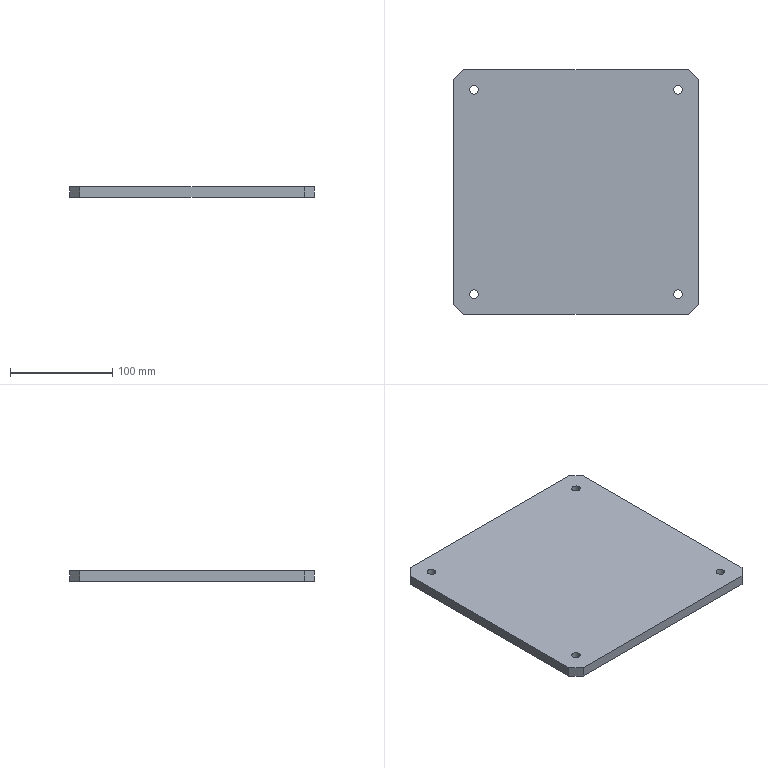Part | STEP file | PN_0011 | 1 solid | 18 faces | box 240 x 240 x 10 mm | volume 571730 mm3 | plane 10 | cylinder 8 | commonest cylinder face diameters 8.5 x8
STEP:
#1=CARTESIAN_POINT('',(0.,0.,0.));
#2=DIRECTION('',(0.,0.,1.));
#3=DIRECTION('',(1.,0.,0.));
#4=AXIS2_PLACEMENT_3D('',#1,#2,#3);
#5=CARTESIAN_POINT('',(-95.75,100.,0.));
#6=VERTEX_POINT('',#5);
#7=CARTESIAN_POINT('',(-95.75,100.,10.));
#8=VERTEX_POINT('',#7);
#9=CARTESIAN_POINT('',(-95.75,100.,10.));
#10=DIRECTION('',(0.,0.,1.));
#11=VECTOR('',#10,1.);
#12=LINE('',#9,#11);
#13=CARTESIAN_POINT('',(-100.,100.,10.));
#14=DIRECTION('',(0.,0.,1.));
#15=DIRECTION('',(1.,0.,0.));
#16=AXIS2_PLACEMENT_3D('',#13,#14,#15);
#17=CYLINDRICAL_SURFACE('',#16,4.25);
#18=CARTESIAN_POINT('',(6.283,0.));
#19=DIRECTION('',(0.,1.));
#20=VECTOR('',#19,1.);
#21=LINE('',#18,#20);
#22=(GEOMETRIC_REPRESENTATION_CONTEXT(2)PARAMETRIC_REPRESENTATION_CONTEXT()REPRESENTATION_CONTEXT('',''));
#23=DEFINITIONAL_REPRESENTATION('',(#21),#22);
#24=PCURVE('',#17,#23);
#25=CARTESIAN_POINT('',(-100.,100.,10.));
#26=DIRECTION('',(0.,0.,1.));
#27=DIRECTION('',(1.,0.,0.));
#28=AXIS2_PLACEMENT_3D('',#25,#26,#27);
#29=CYLINDRICAL_SURFACE('',#28,4.25);
#30=CARTESIAN_POINT('',(0.,0.));
#31=DIRECTION('',(0.,1.));
#32=VECTOR('',#31,1.);
#33=LINE('',#30,#32);
#34=(GEOMETRIC_REPRESENTATION_CONTEXT(2)PARAMETRIC_REPRESENTATION_CONTEXT()REPRESENTATION_CONTEXT('',''));
#35=DEFINITIONAL_REPRESENTATION('',(#33),#34);
#36=PCURVE('',#29,#35);
#37=SURFACE_CURVE('',#12,(#24,#36),.PCURVE_S1.);
#38=EDGE_CURVE('',#6,#8,#37,.T.);
#39=ORIENTED_EDGE('',*,*,#38,.T.);
#40=CARTESIAN_POINT('',(-104.25,100.,10.));
#41=VERTEX_POINT('',#40);
#42=CARTESIAN_POINT('',(-100.,100.,10.));
#43=DIRECTION('',(0.,0.,1.));
#44=DIRECTION('',(1.,0.,0.));
#45=AXIS2_PLACEMENT_3D('',#42,#43,#44);
#46=CIRCLE('',#45,4.25);
#47=CARTESIAN_POINT('',(0.,0.));
#48=DIRECTION('',(1.,0.));
#49=VECTOR('',#48,1.);
#50=LINE('',#47,#49);
#51=(GEOMETRIC_REPRESENTATION_CONTEXT(2)PARAMETRIC_REPRESENTATION_CONTEXT()REPRESENTATION_CONTEXT('',''));
#52=DEFINITIONAL_REPRESENTATION('',(#50),#51);
#53=PCURVE('',#17,#52);
#54=CARTESIAN_POINT('',(0.,0.,10.));
#55=DIRECTION('',(0.,0.,1.));
#56=DIRECTION('',(1.,0.,0.));
#57=AXIS2_PLACEMENT_3D('',#54,#55,#56);
#58=PLANE('',#57);
#59=CARTESIAN_POINT('',(-100.,100.));
#60=DIRECTION('',(1.,0.));
#61=AXIS2_PLACEMENT_2D('',#59,#60);
#62=CIRCLE('',#61,4.25);
#63=(GEOMETRIC_REPRESENTATION_CONTEXT(2)PARAMETRIC_REPRESENTATION_CONTEXT()REPRESENTATION_CONTEXT('',''));
#64=DEFINITIONAL_REPRESENTATION('',(#62),#63);
#65=PCURVE('',#58,#64);
#66=SURFACE_CURVE('',#46,(#53,#65),.PCURVE_S1.);
#67=EDGE_CURVE('',#41,#8,#66,.T.);
#68=ORIENTED_EDGE('',*,*,#67,.F.);
#69=CARTESIAN_POINT('',(-104.25,100.,0.));
#70=VERTEX_POINT('',#69);
#71=CARTESIAN_POINT('',(-104.25,100.,10.));
#72=DIRECTION('',(0.,0.,1.));
#73=VECTOR('',#72,1.);
#74=LINE('',#71,#73);
#75=CARTESIAN_POINT('',(3.142,0.));
#76=DIRECTION('',(0.,1.));
#77=VECTOR('',#76,1.);
#78=LINE('',#75,#77);
#79=(GEOMETRIC_REPRESENTATION_CONTEXT(2)PARAMETRIC_REPRESENTATION_CONTEXT()REPRESENTATION_CONTEXT('',''));
#80=DEFINITIONAL_REPRESENTATION('',(#78),#79);
#81=PCURVE('',#17,#80);
#82=CARTESIAN_POINT('',(3.142,0.));
#83=DIRECTION('',(0.,1.));
#84=VECTOR('',#83,1.);
#85=LINE('',#82,#84);
#86=(GEOMETRIC_REPRESENTATION_CONTEXT(2)PARAMETRIC_REPRESENTATION_CONTEXT()REPRESENTATION_CONTEXT('',''));
#87=DEFINITIONAL_REPRESENTATION('',(#85),#86);
#88=PCURVE('',#29,#87);
#89=SURFACE_CURVE('',#74,(#81,#88),.PCURVE_S1.);
#90=EDGE_CURVE('',#70,#41,#89,.T.);
#91=ORIENTED_EDGE('',*,*,#90,.F.);
#92=CARTESIAN_POINT('',(-100.,100.,0.));
#93=DIRECTION('',(0.,0.,1.));
#94=DIRECTION('',(1.,0.,0.));
#95=AXIS2_PLACEMENT_3D('',#92,#93,#94);
#96=CIRCLE('',#95,4.25);
#97=CARTESIAN_POINT('',(0.,-10.));
#98=DIRECTION('',(1.,0.));
#99=VECTOR('',#98,1.);
#100=LINE('',#97,#99);
#101=(GEOMETRIC_REPRESENTATION_CONTEXT(2)PARAMETRIC_REPRESENTATION_CONTEXT()REPRESENTATION_CONTEXT('',''));
#102=DEFINITIONAL_REPRESENTATION('',(#100),#101);
#103=PCURVE('',#17,#102);
#104=CARTESIAN_POINT('',(0.,0.,0.));
#105=DIRECTION('',(0.,0.,1.));
#106=DIRECTION('',(1.,0.,0.));
#107=AXIS2_PLACEMENT_3D('',#104,#105,#106);
#108=PLANE('',#107);
#109=CARTESIAN_POINT('',(-100.,100.));
#110=DIRECTION('',(1.,0.));
#111=AXIS2_PLACEMENT_2D('',#109,#110);
#112=CIRCLE('',#111,4.25);
#113=(GEOMETRIC_REPRESENTATION_CONTEXT(2)PARAMETRIC_REPRESENTATION_CONTEXT()REPRESENTATION_CONTEXT('',''));
#114=DEFINITIONAL_REPRESENTATION('',(#112),#113);
#115=PCURVE('',#108,#114);
#116=SURFACE_CURVE('',#96,(#103,#115),.PCURVE_S1.);
#117=EDGE_CURVE('',#70,#6,#116,.T.);
#118=ORIENTED_EDGE('',*,*,#117,.T.);
#119=EDGE_LOOP('',(#39,#68,#91,#118));
#120=FACE_BOUND('',#119,.F.);
#121=ADVANCED_FACE('',(#120),#17,.F.);
#122=CARTESIAN_POINT('',(-95.75,-100.,0.));
#123=VERTEX_POINT('',#122);
#124=CARTESIAN_POINT('',(-95.75,-100.,10.));
#125=VERTEX_POINT('',#124);
#126=CARTESIAN_POINT('',(-95.75,-100.,10.));
#127=DIRECTION('',(0.,0.,1.));
#128=VECTOR('',#127,1.);
#129=LINE('',#126,#128);
#130=CARTESIAN_POINT('',(-100.,-100.,10.));
#131=DIRECTION('',(0.,0.,1.));
#132=DIRECTION('',(1.,0.,0.));
#133=AXIS2_PLACEMENT_3D('',#130,#131,#132);
#134=CYLINDRICAL_SURFACE('',#133,4.25);
#135=CARTESIAN_POINT('',(6.283,0.));
#136=DIRECTION('',(0.,1.));
#137=VECTOR('',#136,1.);
#138=LINE('',#135,#137);
#139=(GEOMETRIC_REPRESENTATION_CONTEXT(2)PARAMETRIC_REPRESENTATION_CONTEXT()REPRESENTATION_CONTEXT('',''));
#140=DEFINITIONAL_REPRESENTATION('',(#138),#139);
#141=PCURVE('',#134,#140);
#142=CARTESIAN_POINT('',(-100.,-100.,10.));
#143=DIRECTION('',(0.,0.,1.));
#144=DIRECTION('',(1.,0.,0.));
#145=AXIS2_PLACEMENT_3D('',#142,#143,#144);
#146=CYLINDRICAL_SURFACE('',#145,4.25);
#147=CARTESIAN_POINT('',(0.,0.));
#148=DIRECTION('',(0.,1.));
#149=VECTOR('',#148,1.);
#150=LINE('',#147,#149);
#151=(GEOMETRIC_REPRESENTATION_CONTEXT(2)PARAMETRIC_REPRESENTATION_CONTEXT()REPRESENTATION_CONTEXT('',''));
#152=DEFINITIONAL_REPRESENTATION('',(#150),#151);
#153=PCURVE('',#146,#152);
#154=SURFACE_CURVE('',#129,(#141,#153),.PCURVE_S1.);
#155=EDGE_CURVE('',#123,#125,#154,.T.);
#156=ORIENTED_EDGE('',*,*,#155,.T.);
#157=CARTESIAN_POINT('',(-104.25,-100.,10.));
#158=VERTEX_POINT('',#157);
#159=CARTESIAN_POINT('',(-100.,-100.,10.));
#160=DIRECTION('',(0.,0.,1.));
#161=DIRECTION('',(1.,0.,0.));
#162=AXIS2_PLACEMENT_3D('',#159,#160,#161);
#163=CIRCLE('',#162,4.25);
#164=CARTESIAN_POINT('',(0.,0.));
#165=DIRECTION('',(1.,0.));
#166=VECTOR('',#165,1.);
#167=LINE('',#164,#166);
#168=(GEOMETRIC_REPRESENTATION_CONTEXT(2)PARAMETRIC_REPRESENTATION_CONTEXT()REPRESENTATION_CONTEXT('',''));
#169=DEFINITIONAL_REPRESENTATION('',(#167),#168);
#170=PCURVE('',#134,#169);
#171=CARTESIAN_POINT('',(-100.,-100.));
#172=DIRECTION('',(1.,0.));
#173=AXIS2_PLACEMENT_2D('',#171,#172);
#174=CIRCLE('',#173,4.25);
#175=(GEOMETRIC_REPRESENTATION_CONTEXT(2)PARAMETRIC_REPRESENTATION_CONTEXT()REPRESENTATION_CONTEXT('',''));
#176=DEFINITIONAL_REPRESENTATION('',(#174),#175);
#177=PCURVE('',#58,#176);
#178=SURFACE_CURVE('',#163,(#170,#177),.PCURVE_S1.);
#179=EDGE_CURVE('',#158,#125,#178,.T.);
#180=ORIENTED_EDGE('',*,*,#179,.F.);
#181=CARTESIAN_POINT('',(-104.25,-100.,0.));
#182=VERTEX_POINT('',#181);
#183=CARTESIAN_POINT('',(-104.25,-100.,10.));
#184=DIRECTION('',(0.,0.,1.));
#185=VECTOR('',#184,1.);
#186=LINE('',#183,#185);
#187=CARTESIAN_POINT('',(3.142,0.));
#188=DIRECTION('',(0.,1.));
#189=VECTOR('',#188,1.);
#190=LINE('',#187,#189);
#191=(GEOMETRIC_REPRESENTATION_CONTEXT(2)PARAMETRIC_REPRESENTATION_CONTEXT()REPRESENTATION_CONTEXT('',''));
#192=DEFINITIONAL_REPRESENTATION('',(#190),#191);
#193=PCURVE('',#134,#192);
#194=CARTESIAN_POINT('',(3.142,0.));
#195=DIRECTION('',(0.,1.));
#196=VECTOR('',#195,1.);
#197=LINE('',#194,#196);
#198=(GEOMETRIC_REPRESENTATION_CONTEXT(2)PARAMETRIC_REPRESENTATION_CONTEXT()REPRESENTATION_CONTEXT('',''));
#199=DEFINITIONAL_REPRESENTATION('',(#197),#198);
#200=PCURVE('',#146,#199);
#201=SURFACE_CURVE('',#186,(#193,#200),.PCURVE_S1.);
#202=EDGE_CURVE('',#182,#158,#201,.T.);
#203=ORIENTED_EDGE('',*,*,#202,.F.);
#204=CARTESIAN_POINT('',(-100.,-100.,0.));
#205=DIRECTION('',(0.,0.,1.));
#206=DIRECTION('',(1.,0.,0.));
#207=AXIS2_PLACEMENT_3D('',#204,#205,#206);
#208=CIRCLE('',#207,4.25);
#209=CARTESIAN_POINT('',(0.,-10.));
#210=DIRECTION('',(1.,0.));
#211=VECTOR('',#210,1.);
#212=LINE('',#209,#211);
#213=(GEOMETRIC_REPRESENTATION_CONTEXT(2)PARAMETRIC_REPRESENTATION_CONTEXT()REPRESENTATION_CONTEXT('',''));
#214=DEFINITIONAL_REPRESENTATION('',(#212),#213);
#215=PCURVE('',#134,#214);
#216=CARTESIAN_POINT('',(-100.,-100.));
#217=DIRECTION('',(1.,0.));
#218=AXIS2_PLACEMENT_2D('',#216,#217);
#219=CIRCLE('',#218,4.25);
#220=(GEOMETRIC_REPRESENTATION_CONTEXT(2)PARAMETRIC_REPRESENTATION_CONTEXT()REPRESENTATION_CONTEXT('',''));
#221=DEFINITIONAL_REPRESENTATION('',(#219),#220);
#222=PCURVE('',#108,#221);
#223=SURFACE_CURVE('',#208,(#215,#222),.PCURVE_S1.);
#224=EDGE_CURVE('',#182,#123,#223,.T.);
#225=ORIENTED_EDGE('',*,*,#224,.T.);
#226=EDGE_LOOP('',(#156,#180,#203,#225));
#227=FACE_BOUND('',#226,.F.);
#228=ADVANCED_FACE('',(#227),#134,.F.);
#229=CARTESIAN_POINT('',(104.25,100.,0.));
#230=VERTEX_POINT('',#229);
#231=CARTESIAN_POINT('',(104.25,100.,10.));
#232=VERTEX_POINT('',#231);
#233=CARTESIAN_POINT('',(104.25,100.,10.));
#234=DIRECTION('',(0.,0.,1.));
#235=VECTOR('',#234,1.);
#236=LINE('',#233,#235);
#237=CARTESIAN_POINT('',(100.,100.,10.));
#238=DIRECTION('',(0.,0.,1.));
#239=DIRECTION('',(1.,0.,0.));
#240=AXIS2_PLACEMENT_3D('',#237,#238,#239);
#241=CYLINDRICAL_SURFACE('',#240,4.25);
#242=CARTESIAN_POINT('',(6.283,0.));
#243=DIRECTION('',(0.,1.));
#244=VECTOR('',#243,1.);
#245=LINE('',#242,#244);
#246=(GEOMETRIC_REPRESENTATION_CONTEXT(2)PARAMETRIC_REPRESENTATION_CONTEXT()REPRESENTATION_CONTEXT('',''));
#247=DEFINITIONAL_REPRESENTATION('',(#245),#246);
#248=PCURVE('',#241,#247);
#249=CARTESIAN_POINT('',(100.,100.,10.));
#250=DIRECTION('',(0.,0.,1.));
#251=DIRECTION('',(1.,0.,0.));
#252=AXIS2_PLACEMENT_3D('',#249,#250,#251);
#253=CYLINDRICAL_SURFACE('',#252,4.25);
#254=CARTESIAN_POINT('',(0.,0.));
#255=DIRECTION('',(0.,1.));
#256=VECTOR('',#255,1.);
#257=LINE('',#254,#256);
#258=(GEOMETRIC_REPRESENTATION_CONTEXT(2)PARAMETRIC_REPRESENTATION_CONTEXT()REPRESENTATION_CONTEXT('',''));
#259=DEFINITIONAL_REPRESENTATION('',(#257),#258);
#260=PCURVE('',#253,#259);
#261=SURFACE_CURVE('',#236,(#248,#260),.PCURVE_S1.);
#262=EDGE_CURVE('',#230,#232,#261,.T.);
#263=ORIENTED_EDGE('',*,*,#262,.T.);
#264=CARTESIAN_POINT('',(95.75,100.,10.));
#265=VERTEX_POINT('',#264);
#266=CARTESIAN_POINT('',(100.,100.,10.));
#267=DIRECTION('',(0.,0.,1.));
#268=DIRECTION('',(1.,0.,0.));
#269=AXIS2_PLACEMENT_3D('',#266,#267,#268);
#270=CIRCLE('',#269,4.25);
#271=CARTESIAN_POINT('',(0.,0.));
#272=DIRECTION('',(1.,0.));
#273=VECTOR('',#272,1.);
#274=LINE('',#271,#273);
#275=(GEOMETRIC_REPRESENTATION_CONTEXT(2)PARAMETRIC_REPRESENTATION_CONTEXT()REPRESENTATION_CONTEXT('',''));
#276=DEFINITIONAL_REPRESENTATION('',(#274),#275);
#277=PCURVE('',#241,#276);
#278=CARTESIAN_POINT('',(100.,100.));
#279=DIRECTION('',(1.,0.));
#280=AXIS2_PLACEMENT_2D('',#278,#279);
#281=CIRCLE('',#280,4.25);
#282=(GEOMETRIC_REPRESENTATION_CONTEXT(2)PARAMETRIC_REPRESENTATION_CONTEXT()REPRESENTATION_CONTEXT('',''));
#283=DEFINITIONAL_REPRESENTATION('',(#281),#282);
#284=PCURVE('',#58,#283);
#285=SURFACE_CURVE('',#270,(#277,#284),.PCURVE_S1.);
#286=EDGE_CURVE('',#265,#232,#285,.T.);
#287=ORIENTED_EDGE('',*,*,#286,.F.);
#288=CARTESIAN_POINT('',(95.75,100.,0.));
#289=VERTEX_POINT('',#288);
#290=CARTESIAN_POINT('',(95.75,100.,10.));
#291=DIRECTION('',(0.,0.,1.));
#292=VECTOR('',#291,1.);
#293=LINE('',#290,#292);
#294=CARTESIAN_POINT('',(3.142,0.));
#295=DIRECTION('',(0.,1.));
#296=VECTOR('',#295,1.);
#297=LINE('',#294,#296);
#298=(GEOMETRIC_REPRESENTATION_CONTEXT(2)PARAMETRIC_REPRESENTATION_CONTEXT()REPRESENTATION_CONTEXT('',''));
#299=DEFINITIONAL_REPRESENTATION('',(#297),#298);
#300=PCURVE('',#241,#299);
#301=CARTESIAN_POINT('',(3.142,0.));
#302=DIRECTION('',(0.,1.));
#303=VECTOR('',#302,1.);
#304=LINE('',#301,#303);
#305=(GEOMETRIC_REPRESENTATION_CONTEXT(2)PARAMETRIC_REPRESENTATION_CONTEXT()REPRESENTATION_CONTEXT('',''));
#306=DEFINITIONAL_REPRESENTATION('',(#304),#305);
#307=PCURVE('',#253,#306);
#308=SURFACE_CURVE('',#293,(#300,#307),.PCURVE_S1.);
#309=EDGE_CURVE('',#289,#265,#308,.T.);
#310=ORIENTED_EDGE('',*,*,#309,.F.);
#311=CARTESIAN_POINT('',(100.,100.,0.));
#312=DIRECTION('',(0.,0.,1.));
#313=DIRECTION('',(1.,0.,0.));
#314=AXIS2_PLACEMENT_3D('',#311,#312,#313);
#315=CIRCLE('',#314,4.25);
#316=CARTESIAN_POINT('',(0.,-10.));
#317=DIRECTION('',(1.,0.));
#318=VECTOR('',#317,1.);
#319=LINE('',#316,#318);
#320=(GEOMETRIC_REPRESENTATION_CONTEXT(2)PARAMETRIC_REPRESENTATION_CONTEXT()REPRESENTATION_CONTEXT('',''));
#321=DEFINITIONAL_REPRESENTATION('',(#319),#320);
#322=PCURVE('',#241,#321);
#323=CARTESIAN_POINT('',(100.,100.));
#324=DIRECTION('',(1.,0.));
#325=AXIS2_PLACEMENT_2D('',#323,#324);
#326=CIRCLE('',#325,4.25);
#327=(GEOMETRIC_REPRESENTATION_CONTEXT(2)PARAMETRIC_REPRESENTATION_CONTEXT()REPRESENTATION_CONTEXT('',''));
#328=DEFINITIONAL_REPRESENTATION('',(#326),#327);
#329=PCURVE('',#108,#328);
#330=SURFACE_CURVE('',#315,(#322,#329),.PCURVE_S1.);
#331=EDGE_CURVE('',#289,#230,#330,.T.);
#332=ORIENTED_EDGE('',*,*,#331,.T.);
#333=EDGE_LOOP('',(#263,#287,#310,#332));
#334=FACE_BOUND('',#333,.F.);
#335=ADVANCED_FACE('',(#334),#241,.F.);
#336=CARTESIAN_POINT('',(104.25,-100.,0.));
#337=VERTEX_POINT('',#336);
#338=CARTESIAN_POINT('',(104.25,-100.,10.));
#339=VERTEX_POINT('',#338);
#340=CARTESIAN_POINT('',(104.25,-100.,10.));
#341=DIRECTION('',(0.,0.,1.));
#342=VECTOR('',#341,1.);
#343=LINE('',#340,#342);
#344=CARTESIAN_POINT('',(100.,-100.,10.));
#345=DIRECTION('',(0.,0.,1.));
#346=DIRECTION('',(1.,0.,0.));
#347=AXIS2_PLACEMENT_3D('',#344,#345,#346);
#348=CYLINDRICAL_SURFACE('',#347,4.25);
#349=CARTESIAN_POINT('',(6.283,0.));
#350=DIRECTION('',(0.,1.));
#351=VECTOR('',#350,1.);
#352=LINE('',#349,#351);
#353=(GEOMETRIC_REPRESENTATION_CONTEXT(2)PARAMETRIC_REPRESENTATION_CONTEXT()REPRESENTATION_CONTEXT('',''));
#354=DEFINITIONAL_REPRESENTATION('',(#352),#353);
#355=PCURVE('',#348,#354);
#356=CARTESIAN_POINT('',(100.,-100.,10.));
#357=DIRECTION('',(0.,0.,1.));
#358=DIRECTION('',(1.,0.,0.));
#359=AXIS2_PLACEMENT_3D('',#356,#357,#358);
#360=CYLINDRICAL_SURFACE('',#359,4.25);
#361=CARTESIAN_POINT('',(0.,0.));
#362=DIRECTION('',(0.,1.));
#363=VECTOR('',#362,1.);
#364=LINE('',#361,#363);
#365=(GEOMETRIC_REPRESENTATION_CONTEXT(2)PARAMETRIC_REPRESENTATION_CONTEXT()REPRESENTATION_CONTEXT('',''));
#366=DEFINITIONAL_REPRESENTATION('',(#364),#365);
#367=PCURVE('',#360,#366);
#368=SURFACE_CURVE('',#343,(#355,#367),.PCURVE_S1.);
#369=EDGE_CURVE('',#337,#339,#368,.T.);
#370=ORIENTED_EDGE('',*,*,#369,.T.);
#371=CARTESIAN_POINT('',(95.75,-100.,10.));
#372=VERTEX_POINT('',#371);
#373=CARTESIAN_POINT('',(100.,-100.,10.));
#374=DIRECTION('',(0.,0.,1.));
#375=DIRECTION('',(1.,0.,0.));
#376=AXIS2_PLACEMENT_3D('',#373,#374,#375);
#377=CIRCLE('',#376,4.25);
#378=CARTESIAN_POINT('',(0.,0.));
#379=DIRECTION('',(1.,0.));
#380=VECTOR('',#379,1.);
#381=LINE('',#378,#380);
#382=(GEOMETRIC_REPRESENTATION_CONTEXT(2)PARAMETRIC_REPRESENTATION_CONTEXT()REPRESENTATION_CONTEXT('',''));
#383=DEFINITIONAL_REPRESENTATION('',(#381),#382);
#384=PCURVE('',#348,#383);
#385=CARTESIAN_POINT('',(100.,-100.));
#386=DIRECTION('',(1.,0.));
#387=AXIS2_PLACEMENT_2D('',#385,#386);
#388=CIRCLE('',#387,4.25);
#389=(GEOMETRIC_REPRESENTATION_CONTEXT(2)PARAMETRIC_REPRESENTATION_CONTEXT()REPRESENTATION_CONTEXT('',''));
#390=DEFINITIONAL_REPRESENTATION('',(#388),#389);
#391=PCURVE('',#58,#390);
#392=SURFACE_CURVE('',#377,(#384,#391),.PCURVE_S1.);
#393=EDGE_CURVE('',#372,#339,#392,.T.);
#394=ORIENTED_EDGE('',*,*,#393,.F.);
#395=CARTESIAN_POINT('',(95.75,-100.,0.));
#396=VERTEX_POINT('',#395);
#397=CARTESIAN_POINT('',(95.75,-100.,10.));
#398=DIRECTION('',(0.,0.,1.));
#399=VECTOR('',#398,1.);
#400=LINE('',#397,#399);
#401=CARTESIAN_POINT('',(3.142,0.));
#402=DIRECTION('',(0.,1.));
#403=VECTOR('',#402,1.);
#404=LINE('',#401,#403);
#405=(GEOMETRIC_REPRESENTATION_CONTEXT(2)PARAMETRIC_REPRESENTATION_CONTEXT()REPRESENTATION_CONTEXT('',''));
#406=DEFINITIONAL_REPRESENTATION('',(#404),#405);
#407=PCURVE('',#348,#406);
#408=CARTESIAN_POINT('',(3.142,0.));
#409=DIRECTION('',(0.,1.));
#410=VECTOR('',#409,1.);
#411=LINE('',#408,#410);
#412=(GEOMETRIC_REPRESENTATION_CONTEXT(2)PARAMETRIC_REPRESENTATION_CONTEXT()REPRESENTATION_CONTEXT('',''));
#413=DEFINITIONAL_REPRESENTATION('',(#411),#412);
#414=PCURVE('',#360,#413);
#415=SURFACE_CURVE('',#400,(#407,#414),.PCURVE_S1.);
#416=EDGE_CURVE('',#396,#372,#415,.T.);
#417=ORIENTED_EDGE('',*,*,#416,.F.);
#418=CARTESIAN_POINT('',(100.,-100.,0.));
#419=DIRECTION('',(0.,0.,1.));
#420=DIRECTION('',(1.,0.,0.));
#421=AXIS2_PLACEMENT_3D('',#418,#419,#420);
#422=CIRCLE('',#421,4.25);
#423=CARTESIAN_POINT('',(0.,-10.));
#424=DIRECTION('',(1.,0.));
#425=VECTOR('',#424,1.);
#426=LINE('',#423,#425);
#427=(GEOMETRIC_REPRESENTATION_CONTEXT(2)PARAMETRIC_REPRESENTATION_CONTEXT()REPRESENTATION_CONTEXT('',''));
#428=DEFINITIONAL_REPRESENTATION('',(#426),#427);
#429=PCURVE('',#348,#428);
#430=CARTESIAN_POINT('',(100.,-100.));
#431=DIRECTION('',(1.,0.));
#432=AXIS2_PLACEMENT_2D('',#430,#431);
#433=CIRCLE('',#432,4.25);
#434=(GEOMETRIC_REPRESENTATION_CONTEXT(2)PARAMETRIC_REPRESENTATION_CONTEXT()REPRESENTATION_CONTEXT('',''));
#435=DEFINITIONAL_REPRESENTATION('',(#433),#434);
#436=PCURVE('',#108,#435);
#437=SURFACE_CURVE('',#422,(#429,#436),.PCURVE_S1.);
#438=EDGE_CURVE('',#396,#337,#437,.T.);
#439=ORIENTED_EDGE('',*,*,#438,.T.);
#440=EDGE_LOOP('',(#370,#394,#417,#439));
#441=FACE_BOUND('',#440,.F.);
#442=ADVANCED_FACE('',(#441),#348,.F.);
#443=CARTESIAN_POINT('',(120.,-110.,0.));
#444=VERTEX_POINT('',#443);
#445=CARTESIAN_POINT('',(120.,110.,0.));
#446=VERTEX_POINT('',#445);
#447=CARTESIAN_POINT('',(120.,120.,0.));
#448=DIRECTION('',(0.,1.,0.));
#449=VECTOR('',#448,1.);
#450=LINE('',#447,#449);
#451=CARTESIAN_POINT('',(120.,120.,10.));
#452=DIRECTION('',(-1.,0.,0.));
#453=DIRECTION('',(0.,-1.,0.));
#454=AXIS2_PLACEMENT_3D('',#451,#452,#453);
#455=PLANE('',#454);
#456=CARTESIAN_POINT('',(0.,-10.));
#457=DIRECTION('',(-1.,0.));
#458=VECTOR('',#457,1.);
#459=LINE('',#456,#458);
#460=(GEOMETRIC_REPRESENTATION_CONTEXT(2)PARAMETRIC_REPRESENTATION_CONTEXT()REPRESENTATION_CONTEXT('',''));
#461=DEFINITIONAL_REPRESENTATION('',(#459),#460);
#462=PCURVE('',#455,#461);
#463=CARTESIAN_POINT('',(120.,120.));
#464=DIRECTION('',(0.,1.));
#465=VECTOR('',#464,1.);
#466=LINE('',#463,#465);
#467=(GEOMETRIC_REPRESENTATION_CONTEXT(2)PARAMETRIC_REPRESENTATION_CONTEXT()REPRESENTATION_CONTEXT('',''));
#468=DEFINITIONAL_REPRESENTATION('',(#466),#467);
#469=PCURVE('',#108,#468);
#470=SURFACE_CURVE('',#450,(#462,#469),.PCURVE_S1.);
#471=EDGE_CURVE('',#444,#446,#470,.T.);
#472=ORIENTED_EDGE('',*,*,#471,.T.);
#473=CARTESIAN_POINT('',(120.,110.,10.));
#474=VERTEX_POINT('',#473);
#475=CARTESIAN_POINT('',(120.,110.,10.));
#476=DIRECTION('',(0.,0.,1.));
#477=VECTOR('',#476,1.);
#478=LINE('',#475,#477);
#479=CARTESIAN_POINT('',(10.,0.));
#480=DIRECTION('',(0.,1.));
#481=VECTOR('',#480,1.);
#482=LINE('',#479,#481);
#483=(GEOMETRIC_REPRESENTATION_CONTEXT(2)PARAMETRIC_REPRESENTATION_CONTEXT()REPRESENTATION_CONTEXT('',''));
#484=DEFINITIONAL_REPRESENTATION('',(#482),#483);
#485=PCURVE('',#455,#484);
#486=CARTESIAN_POINT('',(110.,120.,10.));
#487=DIRECTION('',(-0.7071,-0.7071,0.));
#488=DIRECTION('',(0.,0.,-1.));
#489=AXIS2_PLACEMENT_3D('',#486,#487,#488);
#490=PLANE('',#489);
#491=CARTESIAN_POINT('',(0.,14.142));
#492=DIRECTION('',(-1.,0.));
#493=VECTOR('',#492,1.);
#494=LINE('',#491,#493);
#495=(GEOMETRIC_REPRESENTATION_CONTEXT(2)PARAMETRIC_REPRESENTATION_CONTEXT()REPRESENTATION_CONTEXT('',''));
#496=DEFINITIONAL_REPRESENTATION('',(#494),#495);
#497=PCURVE('',#490,#496);
#498=SURFACE_CURVE('',#478,(#485,#497),.PCURVE_S1.);
#499=EDGE_CURVE('',#446,#474,#498,.T.);
#500=ORIENTED_EDGE('',*,*,#499,.T.);
#501=CARTESIAN_POINT('',(120.,-110.,10.));
#502=VERTEX_POINT('',#501);
#503=CARTESIAN_POINT('',(120.,120.,10.));
#504=DIRECTION('',(0.,1.,0.));
#505=VECTOR('',#504,1.);
#506=LINE('',#503,#505);
#507=CARTESIAN_POINT('',(0.,0.));
#508=DIRECTION('',(-1.,0.));
#509=VECTOR('',#508,1.);
#510=LINE('',#507,#509);
#511=(GEOMETRIC_REPRESENTATION_CONTEXT(2)PARAMETRIC_REPRESENTATION_CONTEXT()REPRESENTATION_CONTEXT('',''));
#512=DEFINITIONAL_REPRESENTATION('',(#510),#511);
#513=PCURVE('',#455,#512);
#514=CARTESIAN_POINT('',(120.,120.));
#515=DIRECTION('',(0.,1.));
#516=VECTOR('',#515,1.);
#517=LINE('',#514,#516);
#518=(GEOMETRIC_REPRESENTATION_CONTEXT(2)PARAMETRIC_REPRESENTATION_CONTEXT()REPRESENTATION_CONTEXT('',''));
#519=DEFINITIONAL_REPRESENTATION('',(#517),#518);
#520=PCURVE('',#58,#519);
#521=SURFACE_CURVE('',#506,(#513,#520),.PCURVE_S1.);
#522=EDGE_CURVE('',#502,#474,#521,.T.);
#523=ORIENTED_EDGE('',*,*,#522,.F.);
#524=CARTESIAN_POINT('',(120.,-110.,10.));
#525=DIRECTION('',(0.,0.,-1.));
#526=VECTOR('',#525,1.);
#527=LINE('',#524,#526);
#528=CARTESIAN_POINT('',(230.,0.));
#529=DIRECTION('',(0.,-1.));
#530=VECTOR('',#529,1.);
#531=LINE('',#528,#530);
#532=(GEOMETRIC_REPRESENTATION_CONTEXT(2)PARAMETRIC_REPRESENTATION_CONTEXT()REPRESENTATION_CONTEXT('',''));
#533=DEFINITIONAL_REPRESENTATION('',(#531),#532);
#534=PCURVE('',#455,#533);
#535=CARTESIAN_POINT('',(120.,-110.,10.));
#536=DIRECTION('',(-0.7071,0.7071,0.));
#537=DIRECTION('',(0.,0.,-1.));
#538=AXIS2_PLACEMENT_3D('',#535,#536,#537);
#539=PLANE('',#538);
#540=CARTESIAN_POINT('',(0.,0.));
#541=DIRECTION('',(1.,0.));
#542=VECTOR('',#541,1.);
#543=LINE('',#540,#542);
#544=(GEOMETRIC_REPRESENTATION_CONTEXT(2)PARAMETRIC_REPRESENTATION_CONTEXT()REPRESENTATION_CONTEXT('',''));
#545=DEFINITIONAL_REPRESENTATION('',(#543),#544);
#546=PCURVE('',#539,#545);
#547=SURFACE_CURVE('',#527,(#534,#546),.PCURVE_S1.);
#548=EDGE_CURVE('',#502,#444,#547,.T.);
#549=ORIENTED_EDGE('',*,*,#548,.T.);
#550=EDGE_LOOP('',(#472,#500,#523,#549));
#551=FACE_BOUND('',#550,.T.);
#552=ADVANCED_FACE('',(#551),#455,.F.);
#553=CARTESIAN_POINT('',(110.,120.,10.));
#554=VERTEX_POINT('',#553);
#555=CARTESIAN_POINT('',(-110.,120.,10.));
#556=VERTEX_POINT('',#555);
#557=CARTESIAN_POINT('',(-120.,120.,10.));
#558=DIRECTION('',(-1.,0.,0.));
#559=VECTOR('',#558,1.);
#560=LINE('',#557,#559);
#561=CARTESIAN_POINT('',(-120.,120.,10.));
#562=DIRECTION('',(0.,-1.,0.));
#563=DIRECTION('',(0.,0.,-1.));
#564=AXIS2_PLACEMENT_3D('',#561,#562,#563);
#565=PLANE('',#564);
#566=CARTESIAN_POINT('',(0.,0.));
#567=DIRECTION('',(0.,-1.));
#568=VECTOR('',#567,1.);
#569=LINE('',#566,#568);
#570=(GEOMETRIC_REPRESENTATION_CONTEXT(2)PARAMETRIC_REPRESENTATION_CONTEXT()REPRESENTATION_CONTEXT('',''));
#571=DEFINITIONAL_REPRESENTATION('',(#569),#570);
#572=PCURVE('',#565,#571);
#573=CARTESIAN_POINT('',(-120.,120.));
#574=DIRECTION('',(-1.,0.));
#575=VECTOR('',#574,1.);
#576=LINE('',#573,#575);
#577=(GEOMETRIC_REPRESENTATION_CONTEXT(2)PARAMETRIC_REPRESENTATION_CONTEXT()REPRESENTATION_CONTEXT('',''));
#578=DEFINITIONAL_REPRESENTATION('',(#576),#577);
#579=PCURVE('',#58,#578);
#580=SURFACE_CURVE('',#560,(#572,#579),.PCURVE_S1.);
#581=EDGE_CURVE('',#554,#556,#580,.T.);
#582=ORIENTED_EDGE('',*,*,#581,.F.);
#583=CARTESIAN_POINT('',(110.,120.,0.));
#584=VERTEX_POINT('',#583);
#585=CARTESIAN_POINT('',(110.,120.,10.));
#586=DIRECTION('',(0.,0.,-1.));
#587=VECTOR('',#586,1.);
#588=LINE('',#585,#587);
#589=CARTESIAN_POINT('',(0.,230.));
#590=DIRECTION('',(1.,0.));
#591=VECTOR('',#590,1.);
#592=LINE('',#589,#591);
#593=(GEOMETRIC_REPRESENTATION_CONTEXT(2)PARAMETRIC_REPRESENTATION_CONTEXT()REPRESENTATION_CONTEXT('',''));
#594=DEFINITIONAL_REPRESENTATION('',(#592),#593);
#595=PCURVE('',#565,#594);
#596=CARTESIAN_POINT('',(0.,0.));
#597=DIRECTION('',(1.,0.));
#598=VECTOR('',#597,1.);
#599=LINE('',#596,#598);
#600=(GEOMETRIC_REPRESENTATION_CONTEXT(2)PARAMETRIC_REPRESENTATION_CONTEXT()REPRESENTATION_CONTEXT('',''));
#601=DEFINITIONAL_REPRESENTATION('',(#599),#600);
#602=PCURVE('',#490,#601);
#603=SURFACE_CURVE('',#588,(#595,#602),.PCURVE_S1.);
#604=EDGE_CURVE('',#554,#584,#603,.T.);
#605=ORIENTED_EDGE('',*,*,#604,.T.);
#606=CARTESIAN_POINT('',(-110.,120.,0.));
#607=VERTEX_POINT('',#606);
#608=CARTESIAN_POINT('',(-120.,120.,0.));
#609=DIRECTION('',(-1.,0.,0.));
#610=VECTOR('',#609,1.);
#611=LINE('',#608,#610);
#612=CARTESIAN_POINT('',(10.,0.));
#613=DIRECTION('',(0.,-1.));
#614=VECTOR('',#613,1.);
#615=LINE('',#612,#614);
#616=(GEOMETRIC_REPRESENTATION_CONTEXT(2)PARAMETRIC_REPRESENTATION_CONTEXT()REPRESENTATION_CONTEXT('',''));
#617=DEFINITIONAL_REPRESENTATION('',(#615),#616);
#618=PCURVE('',#565,#617);
#619=CARTESIAN_POINT('',(-120.,120.));
#620=DIRECTION('',(-1.,0.));
#621=VECTOR('',#620,1.);
#622=LINE('',#619,#621);
#623=(GEOMETRIC_REPRESENTATION_CONTEXT(2)PARAMETRIC_REPRESENTATION_CONTEXT()REPRESENTATION_CONTEXT('',''));
#624=DEFINITIONAL_REPRESENTATION('',(#622),#623);
#625=PCURVE('',#108,#624);
#626=SURFACE_CURVE('',#611,(#618,#625),.PCURVE_S1.);
#627=EDGE_CURVE('',#584,#607,#626,.T.);
#628=ORIENTED_EDGE('',*,*,#627,.T.);
#629=CARTESIAN_POINT('',(-110.,120.,10.));
#630=DIRECTION('',(0.,0.,1.));
#631=VECTOR('',#630,1.);
#632=LINE('',#629,#631);
#633=CARTESIAN_POINT('',(0.,10.));
#634=DIRECTION('',(-1.,0.));
#635=VECTOR('',#634,1.);
#636=LINE('',#633,#635);
#637=(GEOMETRIC_REPRESENTATION_CONTEXT(2)PARAMETRIC_REPRESENTATION_CONTEXT()REPRESENTATION_CONTEXT('',''));
#638=DEFINITIONAL_REPRESENTATION('',(#636),#637);
#639=PCURVE('',#565,#638);
#640=CARTESIAN_POINT('',(-120.,110.,10.));
#641=DIRECTION('',(0.7071,-0.7071,0.));
#642=DIRECTION('',(0.,0.,-1.));
#643=AXIS2_PLACEMENT_3D('',#640,#641,#642);
#644=PLANE('',#643);
#645=CARTESIAN_POINT('',(0.,14.142));
#646=DIRECTION('',(-1.,0.));
#647=VECTOR('',#646,1.);
#648=LINE('',#645,#647);
#649=(GEOMETRIC_REPRESENTATION_CONTEXT(2)PARAMETRIC_REPRESENTATION_CONTEXT()REPRESENTATION_CONTEXT('',''));
#650=DEFINITIONAL_REPRESENTATION('',(#648),#649);
#651=PCURVE('',#644,#650);
#652=SURFACE_CURVE('',#632,(#639,#651),.PCURVE_S1.);
#653=EDGE_CURVE('',#607,#556,#652,.T.);
#654=ORIENTED_EDGE('',*,*,#653,.T.);
#655=EDGE_LOOP('',(#582,#605,#628,#654));
#656=FACE_BOUND('',#655,.T.);
#657=ADVANCED_FACE('',(#656),#565,.F.);
#658=CARTESIAN_POINT('',(-120.,110.,10.));
#659=VERTEX_POINT('',#658);
#660=CARTESIAN_POINT('',(-120.,-110.,10.));
#661=VERTEX_POINT('',#660);
#662=CARTESIAN_POINT('',(-120.,120.,10.));
#663=DIRECTION('',(0.,-1.,0.));
#664=VECTOR('',#663,1.);
#665=LINE('',#662,#664);
#666=CARTESIAN_POINT('',(-120.,120.,10.));
#667=DIRECTION('',(1.,0.,0.));
#668=DIRECTION('',(0.,1.,0.));
#669=AXIS2_PLACEMENT_3D('',#666,#667,#668);
#670=PLANE('',#669);
#671=CARTESIAN_POINT('',(0.,0.));
#672=DIRECTION('',(-1.,0.));
#673=VECTOR('',#672,1.);
#674=LINE('',#671,#673);
#675=(GEOMETRIC_REPRESENTATION_CONTEXT(2)PARAMETRIC_REPRESENTATION_CONTEXT()REPRESENTATION_CONTEXT('',''));
#676=DEFINITIONAL_REPRESENTATION('',(#674),#675);
#677=PCURVE('',#670,#676);
#678=CARTESIAN_POINT('',(-120.,120.));
#679=DIRECTION('',(0.,-1.));
#680=VECTOR('',#679,1.);
#681=LINE('',#678,#680);
#682=(GEOMETRIC_REPRESENTATION_CONTEXT(2)PARAMETRIC_REPRESENTATION_CONTEXT()REPRESENTATION_CONTEXT('',''));
#683=DEFINITIONAL_REPRESENTATION('',(#681),#682);
#684=PCURVE('',#58,#683);
#685=SURFACE_CURVE('',#665,(#677,#684),.PCURVE_S1.);
#686=EDGE_CURVE('',#659,#661,#685,.T.);
#687=ORIENTED_EDGE('',*,*,#686,.F.);
#688=CARTESIAN_POINT('',(-120.,110.,0.));
#689=VERTEX_POINT('',#688);
#690=CARTESIAN_POINT('',(-120.,110.,10.));
#691=DIRECTION('',(0.,0.,-1.));
#692=VECTOR('',#691,1.);
#693=LINE('',#690,#692);
#694=CARTESIAN_POINT('',(-10.,0.));
#695=DIRECTION('',(0.,-1.));
#696=VECTOR('',#695,1.);
#697=LINE('',#694,#696);
#698=(GEOMETRIC_REPRESENTATION_CONTEXT(2)PARAMETRIC_REPRESENTATION_CONTEXT()REPRESENTATION_CONTEXT('',''));
#699=DEFINITIONAL_REPRESENTATION('',(#697),#698);
#700=PCURVE('',#670,#699);
#701=CARTESIAN_POINT('',(0.,0.));
#702=DIRECTION('',(1.,0.));
#703=VECTOR('',#702,1.);
#704=LINE('',#701,#703);
#705=(GEOMETRIC_REPRESENTATION_CONTEXT(2)PARAMETRIC_REPRESENTATION_CONTEXT()REPRESENTATION_CONTEXT('',''));
#706=DEFINITIONAL_REPRESENTATION('',(#704),#705);
#707=PCURVE('',#644,#706);
#708=SURFACE_CURVE('',#693,(#700,#707),.PCURVE_S1.);
#709=EDGE_CURVE('',#659,#689,#708,.T.);
#710=ORIENTED_EDGE('',*,*,#709,.T.);
#711=CARTESIAN_POINT('',(-120.,-110.,0.));
#712=VERTEX_POINT('',#711);
#713=CARTESIAN_POINT('',(-120.,120.,0.));
#714=DIRECTION('',(0.,-1.,0.));
#715=VECTOR('',#714,1.);
#716=LINE('',#713,#715);
#717=CARTESIAN_POINT('',(0.,-10.));
#718=DIRECTION('',(-1.,0.));
#719=VECTOR('',#718,1.);
#720=LINE('',#717,#719);
#721=(GEOMETRIC_REPRESENTATION_CONTEXT(2)PARAMETRIC_REPRESENTATION_CONTEXT()REPRESENTATION_CONTEXT('',''));
#722=DEFINITIONAL_REPRESENTATION('',(#720),#721);
#723=PCURVE('',#670,#722);
#724=CARTESIAN_POINT('',(-120.,120.));
#725=DIRECTION('',(0.,-1.));
#726=VECTOR('',#725,1.);
#727=LINE('',#724,#726);
#728=(GEOMETRIC_REPRESENTATION_CONTEXT(2)PARAMETRIC_REPRESENTATION_CONTEXT()REPRESENTATION_CONTEXT('',''));
#729=DEFINITIONAL_REPRESENTATION('',(#727),#728);
#730=PCURVE('',#108,#729);
#731=SURFACE_CURVE('',#716,(#723,#730),.PCURVE_S1.);
#732=EDGE_CURVE('',#689,#712,#731,.T.);
#733=ORIENTED_EDGE('',*,*,#732,.T.);
#734=CARTESIAN_POINT('',(-120.,-110.,10.));
#735=DIRECTION('',(0.,0.,1.));
#736=VECTOR('',#735,1.);
#737=LINE('',#734,#736);
#738=CARTESIAN_POINT('',(-230.,0.));
#739=DIRECTION('',(0.,1.));
#740=VECTOR('',#739,1.);
#741=LINE('',#738,#740);
#742=(GEOMETRIC_REPRESENTATION_CONTEXT(2)PARAMETRIC_REPRESENTATION_CONTEXT()REPRESENTATION_CONTEXT('',''));
#743=DEFINITIONAL_REPRESENTATION('',(#741),#742);
#744=PCURVE('',#670,#743);
#745=CARTESIAN_POINT('',(-110.,-120.,10.));
#746=DIRECTION('',(0.7071,0.7071,0.));
#747=DIRECTION('',(0.,0.,-1.));
#748=AXIS2_PLACEMENT_3D('',#745,#746,#747);
#749=PLANE('',#748);
#750=CARTESIAN_POINT('',(0.,14.142));
#751=DIRECTION('',(-1.,0.));
#752=VECTOR('',#751,1.);
#753=LINE('',#750,#752);
#754=(GEOMETRIC_REPRESENTATION_CONTEXT(2)PARAMETRIC_REPRESENTATION_CONTEXT()REPRESENTATION_CONTEXT('',''));
#755=DEFINITIONAL_REPRESENTATION('',(#753),#754);
#756=PCURVE('',#749,#755);
#757=SURFACE_CURVE('',#737,(#744,#756),.PCURVE_S1.);
#758=EDGE_CURVE('',#712,#661,#757,.T.);
#759=ORIENTED_EDGE('',*,*,#758,.T.);
#760=EDGE_LOOP('',(#687,#710,#733,#759));
#761=FACE_BOUND('',#760,.T.);
#762=ADVANCED_FACE('',(#761),#670,.F.);
#763=CARTESIAN_POINT('',(-110.,-120.,10.));
#764=VERTEX_POINT('',#763);
#765=CARTESIAN_POINT('',(110.,-120.,10.));
#766=VERTEX_POINT('',#765);
#767=CARTESIAN_POINT('',(-120.,-120.,10.));
#768=DIRECTION('',(1.,0.,0.));
#769=VECTOR('',#768,1.);
#770=LINE('',#767,#769);
#771=CARTESIAN_POINT('',(-120.,-120.,10.));
#772=DIRECTION('',(0.,1.,0.));
#773=DIRECTION('',(0.,0.,1.));
#774=AXIS2_PLACEMENT_3D('',#771,#772,#773);
#775=PLANE('',#774);
#776=CARTESIAN_POINT('',(0.,0.));
#777=DIRECTION('',(0.,1.));
#778=VECTOR('',#777,1.);
#779=LINE('',#776,#778);
#780=(GEOMETRIC_REPRESENTATION_CONTEXT(2)PARAMETRIC_REPRESENTATION_CONTEXT()REPRESENTATION_CONTEXT('',''));
#781=DEFINITIONAL_REPRESENTATION('',(#779),#780);
#782=PCURVE('',#775,#781);
#783=CARTESIAN_POINT('',(-120.,-120.));
#784=DIRECTION('',(1.,0.));
#785=VECTOR('',#784,1.);
#786=LINE('',#783,#785);
#787=(GEOMETRIC_REPRESENTATION_CONTEXT(2)PARAMETRIC_REPRESENTATION_CONTEXT()REPRESENTATION_CONTEXT('',''));
#788=DEFINITIONAL_REPRESENTATION('',(#786),#787);
#789=PCURVE('',#58,#788);
#790=SURFACE_CURVE('',#770,(#782,#789),.PCURVE_S1.);
#791=EDGE_CURVE('',#764,#766,#790,.T.);
#792=ORIENTED_EDGE('',*,*,#791,.F.);
#793=CARTESIAN_POINT('',(-110.,-120.,0.));
#794=VERTEX_POINT('',#793);
#795=CARTESIAN_POINT('',(-110.,-120.,10.));
#796=DIRECTION('',(0.,0.,-1.));
#797=VECTOR('',#796,1.);
#798=LINE('',#795,#797);
#799=CARTESIAN_POINT('',(0.,10.));
#800=DIRECTION('',(-1.,0.));
#801=VECTOR('',#800,1.);
#802=LINE('',#799,#801);
#803=(GEOMETRIC_REPRESENTATION_CONTEXT(2)PARAMETRIC_REPRESENTATION_CONTEXT()REPRESENTATION_CONTEXT('',''));
#804=DEFINITIONAL_REPRESENTATION('',(#802),#803);
#805=PCURVE('',#775,#804);
#806=CARTESIAN_POINT('',(0.,0.));
#807=DIRECTION('',(1.,0.));
#808=VECTOR('',#807,1.);
#809=LINE('',#806,#808);
#810=(GEOMETRIC_REPRESENTATION_CONTEXT(2)PARAMETRIC_REPRESENTATION_CONTEXT()REPRESENTATION_CONTEXT('',''));
#811=DEFINITIONAL_REPRESENTATION('',(#809),#810);
#812=PCURVE('',#749,#811);
#813=SURFACE_CURVE('',#798,(#805,#812),.PCURVE_S1.);
#814=EDGE_CURVE('',#764,#794,#813,.T.);
#815=ORIENTED_EDGE('',*,*,#814,.T.);
#816=CARTESIAN_POINT('',(110.,-120.,0.));
#817=VERTEX_POINT('',#816);
#818=CARTESIAN_POINT('',(-120.,-120.,0.));
#819=DIRECTION('',(1.,0.,0.));
#820=VECTOR('',#819,1.);
#821=LINE('',#818,#820);
#822=CARTESIAN_POINT('',(-10.,0.));
#823=DIRECTION('',(0.,1.));
#824=VECTOR('',#823,1.);
#825=LINE('',#822,#824);
#826=(GEOMETRIC_REPRESENTATION_CONTEXT(2)PARAMETRIC_REPRESENTATION_CONTEXT()REPRESENTATION_CONTEXT('',''));
#827=DEFINITIONAL_REPRESENTATION('',(#825),#826);
#828=PCURVE('',#775,#827);
#829=CARTESIAN_POINT('',(-120.,-120.));
#830=DIRECTION('',(1.,0.));
#831=VECTOR('',#830,1.);
#832=LINE('',#829,#831);
#833=(GEOMETRIC_REPRESENTATION_CONTEXT(2)PARAMETRIC_REPRESENTATION_CONTEXT()REPRESENTATION_CONTEXT('',''));
#834=DEFINITIONAL_REPRESENTATION('',(#832),#833);
#835=PCURVE('',#108,#834);
#836=SURFACE_CURVE('',#821,(#828,#835),.PCURVE_S1.);
#837=EDGE_CURVE('',#794,#817,#836,.T.);
#838=ORIENTED_EDGE('',*,*,#837,.T.);
#839=CARTESIAN_POINT('',(110.,-120.,10.));
#840=DIRECTION('',(0.,0.,1.));
#841=VECTOR('',#840,1.);
#842=LINE('',#839,#841);
#843=CARTESIAN_POINT('',(0.,230.));
#844=DIRECTION('',(1.,0.));
#845=VECTOR('',#844,1.);
#846=LINE('',#843,#845);
#847=(GEOMETRIC_REPRESENTATION_CONTEXT(2)PARAMETRIC_REPRESENTATION_CONTEXT()REPRESENTATION_CONTEXT('',''));
#848=DEFINITIONAL_REPRESENTATION('',(#846),#847);
#849=PCURVE('',#775,#848);
#850=CARTESIAN_POINT('',(0.,14.142));
#851=DIRECTION('',(-1.,0.));
#852=VECTOR('',#851,1.);
#853=LINE('',#850,#852);
#854=(GEOMETRIC_REPRESENTATION_CONTEXT(2)PARAMETRIC_REPRESENTATION_CONTEXT()REPRESENTATION_CONTEXT('',''));
#855=DEFINITIONAL_REPRESENTATION('',(#853),#854);
#856=PCURVE('',#539,#855);
#857=SURFACE_CURVE('',#842,(#849,#856),.PCURVE_S1.);
#858=EDGE_CURVE('',#817,#766,#857,.T.);
#859=ORIENTED_EDGE('',*,*,#858,.T.);
#860=EDGE_LOOP('',(#792,#815,#838,#859));
#861=FACE_BOUND('',#860,.T.);
#862=ADVANCED_FACE('',(#861),#775,.F.);
#863=CARTESIAN_POINT('',(-100.,100.,10.));
#864=DIRECTION('',(0.,0.,1.));
#865=DIRECTION('',(1.,0.,0.));
#866=AXIS2_PLACEMENT_3D('',#863,#864,#865);
#867=CIRCLE('',#866,4.25);
#868=CARTESIAN_POINT('',(-100.,100.));
#869=DIRECTION('',(1.,0.));
#870=AXIS2_PLACEMENT_2D('',#868,#869);
#871=CIRCLE('',#870,4.25);
#872=(GEOMETRIC_REPRESENTATION_CONTEXT(2)PARAMETRIC_REPRESENTATION_CONTEXT()REPRESENTATION_CONTEXT('',''));
#873=DEFINITIONAL_REPRESENTATION('',(#871),#872);
#874=PCURVE('',#58,#873);
#875=CARTESIAN_POINT('',(0.,0.));
#876=DIRECTION('',(1.,0.));
#877=VECTOR('',#876,1.);
#878=LINE('',#875,#877);
#879=(GEOMETRIC_REPRESENTATION_CONTEXT(2)PARAMETRIC_REPRESENTATION_CONTEXT()REPRESENTATION_CONTEXT('',''));
#880=DEFINITIONAL_REPRESENTATION('',(#878),#879);
#881=PCURVE('',#29,#880);
#882=SURFACE_CURVE('',#867,(#874,#881),.PCURVE_S1.);
#883=EDGE_CURVE('',#8,#41,#882,.T.);
#884=ORIENTED_EDGE('',*,*,#883,.F.);
#885=ORIENTED_EDGE('',*,*,#67,.F.);
#886=EDGE_LOOP('',(#884,#885));
#887=FACE_BOUND('',#886,.T.);
#888=CARTESIAN_POINT('',(-100.,-100.,10.));
#889=DIRECTION('',(0.,0.,1.));
#890=DIRECTION('',(1.,0.,0.));
#891=AXIS2_PLACEMENT_3D('',#888,#889,#890);
#892=CIRCLE('',#891,4.25);
#893=CARTESIAN_POINT('',(-100.,-100.));
#894=DIRECTION('',(1.,0.));
#895=AXIS2_PLACEMENT_2D('',#893,#894);
#896=CIRCLE('',#895,4.25);
#897=(GEOMETRIC_REPRESENTATION_CONTEXT(2)PARAMETRIC_REPRESENTATION_CONTEXT()REPRESENTATION_CONTEXT('',''));
#898=DEFINITIONAL_REPRESENTATION('',(#896),#897);
#899=PCURVE('',#58,#898);
#900=CARTESIAN_POINT('',(0.,0.));
#901=DIRECTION('',(1.,0.));
#902=VECTOR('',#901,1.);
#903=LINE('',#900,#902);
#904=(GEOMETRIC_REPRESENTATION_CONTEXT(2)PARAMETRIC_REPRESENTATION_CONTEXT()REPRESENTATION_CONTEXT('',''));
#905=DEFINITIONAL_REPRESENTATION('',(#903),#904);
#906=PCURVE('',#146,#905);
#907=SURFACE_CURVE('',#892,(#899,#906),.PCURVE_S1.);
#908=EDGE_CURVE('',#125,#158,#907,.T.);
#909=ORIENTED_EDGE('',*,*,#908,.F.);
#910=ORIENTED_EDGE('',*,*,#179,.F.);
#911=EDGE_LOOP('',(#909,#910));
#912=FACE_BOUND('',#911,.T.);
#913=CARTESIAN_POINT('',(100.,100.,10.));
#914=DIRECTION('',(0.,0.,1.));
#915=DIRECTION('',(1.,0.,0.));
#916=AXIS2_PLACEMENT_3D('',#913,#914,#915);
#917=CIRCLE('',#916,4.25);
#918=CARTESIAN_POINT('',(100.,100.));
#919=DIRECTION('',(1.,0.));
#920=AXIS2_PLACEMENT_2D('',#918,#919);
#921=CIRCLE('',#920,4.25);
#922=(GEOMETRIC_REPRESENTATION_CONTEXT(2)PARAMETRIC_REPRESENTATION_CONTEXT()REPRESENTATION_CONTEXT('',''));
#923=DEFINITIONAL_REPRESENTATION('',(#921),#922);
#924=PCURVE('',#58,#923);
#925=CARTESIAN_POINT('',(0.,0.));
#926=DIRECTION('',(1.,0.));
#927=VECTOR('',#926,1.);
#928=LINE('',#925,#927);
#929=(GEOMETRIC_REPRESENTATION_CONTEXT(2)PARAMETRIC_REPRESENTATION_CONTEXT()REPRESENTATION_CONTEXT('',''));
#930=DEFINITIONAL_REPRESENTATION('',(#928),#929);
#931=PCURVE('',#253,#930);
#932=SURFACE_CURVE('',#917,(#924,#931),.PCURVE_S1.);
#933=EDGE_CURVE('',#232,#265,#932,.T.);
#934=ORIENTED_EDGE('',*,*,#933,.F.);
#935=ORIENTED_EDGE('',*,*,#286,.F.);
#936=EDGE_LOOP('',(#934,#935));
#937=FACE_BOUND('',#936,.T.);
#938=CARTESIAN_POINT('',(100.,-100.,10.));
#939=DIRECTION('',(0.,0.,1.));
#940=DIRECTION('',(1.,0.,0.));
#941=AXIS2_PLACEMENT_3D('',#938,#939,#940);
#942=CIRCLE('',#941,4.25);
#943=CARTESIAN_POINT('',(100.,-100.));
#944=DIRECTION('',(1.,0.));
#945=AXIS2_PLACEMENT_2D('',#943,#944);
#946=CIRCLE('',#945,4.25);
#947=(GEOMETRIC_REPRESENTATION_CONTEXT(2)PARAMETRIC_REPRESENTATION_CONTEXT()REPRESENTATION_CONTEXT('',''));
#948=DEFINITIONAL_REPRESENTATION('',(#946),#947);
#949=PCURVE('',#58,#948);
#950=CARTESIAN_POINT('',(0.,0.));
#951=DIRECTION('',(1.,0.));
#952=VECTOR('',#951,1.);
#953=LINE('',#950,#952);
#954=(GEOMETRIC_REPRESENTATION_CONTEXT(2)PARAMETRIC_REPRESENTATION_CONTEXT()REPRESENTATION_CONTEXT('',''));
#955=DEFINITIONAL_REPRESENTATION('',(#953),#954);
#956=PCURVE('',#360,#955);
#957=SURFACE_CURVE('',#942,(#949,#956),.PCURVE_S1.);
#958=EDGE_CURVE('',#339,#372,#957,.T.);
#959=ORIENTED_EDGE('',*,*,#958,.F.);
#960=ORIENTED_EDGE('',*,*,#393,.F.);
#961=EDGE_LOOP('',(#959,#960));
#962=FACE_BOUND('',#961,.T.);
#963=ORIENTED_EDGE('',*,*,#522,.T.);
#964=CARTESIAN_POINT('',(115.,115.,10.));
#965=DIRECTION('',(-0.7071,0.7071,0.));
#966=VECTOR('',#965,1.);
#967=LINE('',#964,#966);
#968=CARTESIAN_POINT('',(115.,115.));
#969=DIRECTION('',(-0.7071,0.7071));
#970=VECTOR('',#969,1.);
#971=LINE('',#968,#970);
#972=(GEOMETRIC_REPRESENTATION_CONTEXT(2)PARAMETRIC_REPRESENTATION_CONTEXT()REPRESENTATION_CONTEXT('',''));
#973=DEFINITIONAL_REPRESENTATION('',(#971),#972);
#974=PCURVE('',#58,#973);
#975=CARTESIAN_POINT('',(0.,7.071));
#976=DIRECTION('',(0.,-1.));
#977=VECTOR('',#976,1.);
#978=LINE('',#975,#977);
#979=(GEOMETRIC_REPRESENTATION_CONTEXT(2)PARAMETRIC_REPRESENTATION_CONTEXT()REPRESENTATION_CONTEXT('',''));
#980=DEFINITIONAL_REPRESENTATION('',(#978),#979);
#981=PCURVE('',#490,#980);
#982=SURFACE_CURVE('',#967,(#974,#981),.PCURVE_S1.);
#983=EDGE_CURVE('',#474,#554,#982,.T.);
#984=ORIENTED_EDGE('',*,*,#983,.T.);
#985=ORIENTED_EDGE('',*,*,#581,.T.);
#986=CARTESIAN_POINT('',(-115.,115.,10.));
#987=DIRECTION('',(-0.7071,-0.7071,0.));
#988=VECTOR('',#987,1.);
#989=LINE('',#986,#988);
#990=CARTESIAN_POINT('',(-115.,115.));
#991=DIRECTION('',(-0.7071,-0.7071));
#992=VECTOR('',#991,1.);
#993=LINE('',#990,#992);
#994=(GEOMETRIC_REPRESENTATION_CONTEXT(2)PARAMETRIC_REPRESENTATION_CONTEXT()REPRESENTATION_CONTEXT('',''));
#995=DEFINITIONAL_REPRESENTATION('',(#993),#994);
#996=PCURVE('',#58,#995);
#997=CARTESIAN_POINT('',(0.,7.071));
#998=DIRECTION('',(0.,-1.));
#999=VECTOR('',#998,1.);
#1000=LINE('',#997,#999);
#1001=(GEOMETRIC_REPRESENTATION_CONTEXT(2)PARAMETRIC_REPRESENTATION_CONTEXT()REPRESENTATION_CONTEXT('',''));
#1002=DEFINITIONAL_REPRESENTATION('',(#1000),#1001);
#1003=PCURVE('',#644,#1002);
#1004=SURFACE_CURVE('',#989,(#996,#1003),.PCURVE_S1.);
#1005=EDGE_CURVE('',#556,#659,#1004,.T.);
#1006=ORIENTED_EDGE('',*,*,#1005,.T.);
#1007=ORIENTED_EDGE('',*,*,#686,.T.);
#1008=CARTESIAN_POINT('',(-115.,-115.,10.));
#1009=DIRECTION('',(0.7071,-0.7071,0.));
#1010=VECTOR('',#1009,1.);
#1011=LINE('',#1008,#1010);
#1012=CARTESIAN_POINT('',(-115.,-115.));
#1013=DIRECTION('',(0.7071,-0.7071));
#1014=VECTOR('',#1013,1.);
#1015=LINE('',#1012,#1014);
#1016=(GEOMETRIC_REPRESENTATION_CONTEXT(2)PARAMETRIC_REPRESENTATION_CONTEXT()REPRESENTATION_CONTEXT('',''));
#1017=DEFINITIONAL_REPRESENTATION('',(#1015),#1016);
#1018=PCURVE('',#58,#1017);
#1019=CARTESIAN_POINT('',(0.,7.071));
#1020=DIRECTION('',(0.,-1.));
#1021=VECTOR('',#1020,1.);
#1022=LINE('',#1019,#1021);
#1023=(GEOMETRIC_REPRESENTATION_CONTEXT(2)PARAMETRIC_REPRESENTATION_CONTEXT()REPRESENTATION_CONTEXT('',''));
#1024=DEFINITIONAL_REPRESENTATION('',(#1022),#1023);
#1025=PCURVE('',#749,#1024);
#1026=SURFACE_CURVE('',#1011,(#1018,#1025),.PCURVE_S1.);
#1027=EDGE_CURVE('',#661,#764,#1026,.T.);
#1028=ORIENTED_EDGE('',*,*,#1027,.T.);
#1029=ORIENTED_EDGE('',*,*,#791,.T.);
#1030=CARTESIAN_POINT('',(115.,-115.,10.));
#1031=DIRECTION('',(0.7071,0.7071,0.));
#1032=VECTOR('',#1031,1.);
#1033=LINE('',#1030,#1032);
#1034=CARTESIAN_POINT('',(115.,-115.));
#1035=DIRECTION('',(0.7071,0.7071));
#1036=VECTOR('',#1035,1.);
#1037=LINE('',#1034,#1036);
#1038=(GEOMETRIC_REPRESENTATION_CONTEXT(2)PARAMETRIC_REPRESENTATION_CONTEXT()REPRESENTATION_CONTEXT('',''));
#1039=DEFINITIONAL_REPRESENTATION('',(#1037),#1038);
#1040=PCURVE('',#58,#1039);
#1041=CARTESIAN_POINT('',(0.,7.071));
#1042=DIRECTION('',(0.,-1.));
#1043=VECTOR('',#1042,1.);
#1044=LINE('',#1041,#1043);
#1045=(GEOMETRIC_REPRESENTATION_CONTEXT(2)PARAMETRIC_REPRESENTATION_CONTEXT()REPRESENTATION_CONTEXT('',''));
#1046=DEFINITIONAL_REPRESENTATION('',(#1044),#1045);
#1047=PCURVE('',#539,#1046);
#1048=SURFACE_CURVE('',#1033,(#1040,#1047),.PCURVE_S1.);
#1049=EDGE_CURVE('',#766,#502,#1048,.T.);
#1050=ORIENTED_EDGE('',*,*,#1049,.T.);
#1051=EDGE_LOOP('',(#963,#984,#985,#1006,#1007,#1028,#1029,#1050));
#1052=FACE_BOUND('',#1051,.T.);
#1053=ADVANCED_FACE('',(#887,#912,#937,#962,#1052),#58,.T.);
#1054=CARTESIAN_POINT('',(-100.,100.,0.));
#1055=DIRECTION('',(0.,0.,1.));
#1056=DIRECTION('',(1.,0.,0.));
#1057=AXIS2_PLACEMENT_3D('',#1054,#1055,#1056);
#1058=CIRCLE('',#1057,4.25);
#1059=CARTESIAN_POINT('',(-100.,100.));
#1060=DIRECTION('',(1.,0.));
#1061=AXIS2_PLACEMENT_2D('',#1059,#1060);
#1062=CIRCLE('',#1061,4.25);
#1063=(GEOMETRIC_REPRESENTATION_CONTEXT(2)PARAMETRIC_REPRESENTATION_CONTEXT()REPRESENTATION_CONTEXT('',''));
#1064=DEFINITIONAL_REPRESENTATION('',(#1062),#1063);
#1065=PCURVE('',#108,#1064);
#1066=CARTESIAN_POINT('',(0.,-10.));
#1067=DIRECTION('',(1.,0.));
#1068=VECTOR('',#1067,1.);
#1069=LINE('',#1066,#1068);
#1070=(GEOMETRIC_REPRESENTATION_CONTEXT(2)PARAMETRIC_REPRESENTATION_CONTEXT()REPRESENTATION_CONTEXT('',''));
#1071=DEFINITIONAL_REPRESENTATION('',(#1069),#1070);
#1072=PCURVE('',#29,#1071);
#1073=SURFACE_CURVE('',#1058,(#1065,#1072),.PCURVE_S1.);
#1074=EDGE_CURVE('',#6,#70,#1073,.T.);
#1075=ORIENTED_EDGE('',*,*,#1074,.T.);
#1076=ORIENTED_EDGE('',*,*,#117,.T.);
#1077=EDGE_LOOP('',(#1075,#1076));
#1078=FACE_BOUND('',#1077,.T.);
#1079=CARTESIAN_POINT('',(-100.,-100.,0.));
#1080=DIRECTION('',(0.,0.,1.));
#1081=DIRECTION('',(1.,0.,0.));
#1082=AXIS2_PLACEMENT_3D('',#1079,#1080,#1081);
#1083=CIRCLE('',#1082,4.25);
#1084=CARTESIAN_POINT('',(-100.,-100.));
#1085=DIRECTION('',(1.,0.));
#1086=AXIS2_PLACEMENT_2D('',#1084,#1085);
#1087=CIRCLE('',#1086,4.25);
#1088=(GEOMETRIC_REPRESENTATION_CONTEXT(2)PARAMETRIC_REPRESENTATION_CONTEXT()REPRESENTATION_CONTEXT('',''));
#1089=DEFINITIONAL_REPRESENTATION('',(#1087),#1088);
#1090=PCURVE('',#108,#1089);
#1091=CARTESIAN_POINT('',(0.,-10.));
#1092=DIRECTION('',(1.,0.));
#1093=VECTOR('',#1092,1.);
#1094=LINE('',#1091,#1093);
#1095=(GEOMETRIC_REPRESENTATION_CONTEXT(2)PARAMETRIC_REPRESENTATION_CONTEXT()REPRESENTATION_CONTEXT('',''));
#1096=DEFINITIONAL_REPRESENTATION('',(#1094),#1095);
#1097=PCURVE('',#146,#1096);
#1098=SURFACE_CURVE('',#1083,(#1090,#1097),.PCURVE_S1.);
#1099=EDGE_CURVE('',#123,#182,#1098,.T.);
#1100=ORIENTED_EDGE('',*,*,#1099,.T.);
#1101=ORIENTED_EDGE('',*,*,#224,.T.);
#1102=EDGE_LOOP('',(#1100,#1101));
#1103=FACE_BOUND('',#1102,.T.);
#1104=CARTESIAN_POINT('',(100.,100.,0.));
#1105=DIRECTION('',(0.,0.,1.));
#1106=DIRECTION('',(1.,0.,0.));
#1107=AXIS2_PLACEMENT_3D('',#1104,#1105,#1106);
#1108=CIRCLE('',#1107,4.25);
#1109=CARTESIAN_POINT('',(100.,100.));
#1110=DIRECTION('',(1.,0.));
#1111=AXIS2_PLACEMENT_2D('',#1109,#1110);
#1112=CIRCLE('',#1111,4.25);
#1113=(GEOMETRIC_REPRESENTATION_CONTEXT(2)PARAMETRIC_REPRESENTATION_CONTEXT()REPRESENTATION_CONTEXT('',''));
#1114=DEFINITIONAL_REPRESENTATION('',(#1112),#1113);
#1115=PCURVE('',#108,#1114);
#1116=CARTESIAN_POINT('',(0.,-10.));
#1117=DIRECTION('',(1.,0.));
#1118=VECTOR('',#1117,1.);
#1119=LINE('',#1116,#1118);
#1120=(GEOMETRIC_REPRESENTATION_CONTEXT(2)PARAMETRIC_REPRESENTATION_CONTEXT()REPRESENTATION_CONTEXT('',''));
#1121=DEFINITIONAL_REPRESENTATION('',(#1119),#1120);
#1122=PCURVE('',#253,#1121);
#1123=SURFACE_CURVE('',#1108,(#1115,#1122),.PCURVE_S1.);
#1124=EDGE_CURVE('',#230,#289,#1123,.T.);
#1125=ORIENTED_EDGE('',*,*,#1124,.T.);
#1126=ORIENTED_EDGE('',*,*,#331,.T.);
#1127=EDGE_LOOP('',(#1125,#1126));
#1128=FACE_BOUND('',#1127,.T.);
#1129=CARTESIAN_POINT('',(100.,-100.,0.));
#1130=DIRECTION('',(0.,0.,1.));
#1131=DIRECTION('',(1.,0.,0.));
#1132=AXIS2_PLACEMENT_3D('',#1129,#1130,#1131);
#1133=CIRCLE('',#1132,4.25);
#1134=CARTESIAN_POINT('',(100.,-100.));
#1135=DIRECTION('',(1.,0.));
#1136=AXIS2_PLACEMENT_2D('',#1134,#1135);
#1137=CIRCLE('',#1136,4.25);
#1138=(GEOMETRIC_REPRESENTATION_CONTEXT(2)PARAMETRIC_REPRESENTATION_CONTEXT()REPRESENTATION_CONTEXT('',''));
#1139=DEFINITIONAL_REPRESENTATION('',(#1137),#1138);
#1140=PCURVE('',#108,#1139);
#1141=CARTESIAN_POINT('',(0.,-10.));
#1142=DIRECTION('',(1.,0.));
#1143=VECTOR('',#1142,1.);
#1144=LINE('',#1141,#1143);
#1145=(GEOMETRIC_REPRESENTATION_CONTEXT(2)PARAMETRIC_REPRESENTATION_CONTEXT()REPRESENTATION_CONTEXT('',''));
#1146=DEFINITIONAL_REPRESENTATION('',(#1144),#1145);
#1147=PCURVE('',#360,#1146);
#1148=SURFACE_CURVE('',#1133,(#1140,#1147),.PCURVE_S1.);
#1149=EDGE_CURVE('',#337,#396,#1148,.T.);
#1150=ORIENTED_EDGE('',*,*,#1149,.T.);
#1151=ORIENTED_EDGE('',*,*,#438,.T.);
#1152=EDGE_LOOP('',(#1150,#1151));
#1153=FACE_BOUND('',#1152,.T.);
#1154=ORIENTED_EDGE('',*,*,#627,.F.);
#1155=CARTESIAN_POINT('',(110.,120.,0.));
#1156=DIRECTION('',(0.7071,-0.7071,0.));
#1157=VECTOR('',#1156,1.);
#1158=LINE('',#1155,#1157);
#1159=CARTESIAN_POINT('',(110.,120.));
#1160=DIRECTION('',(0.7071,-0.7071));
#1161=VECTOR('',#1160,1.);
#1162=LINE('',#1159,#1161);
#1163=(GEOMETRIC_REPRESENTATION_CONTEXT(2)PARAMETRIC_REPRESENTATION_CONTEXT()REPRESENTATION_CONTEXT('',''));
#1164=DEFINITIONAL_REPRESENTATION('',(#1162),#1163);
#1165=PCURVE('',#108,#1164);
#1166=CARTESIAN_POINT('',(10.,0.));
#1167=DIRECTION('',(0.,1.));
#1168=VECTOR('',#1167,1.);
#1169=LINE('',#1166,#1168);
#1170=(GEOMETRIC_REPRESENTATION_CONTEXT(2)PARAMETRIC_REPRESENTATION_CONTEXT()REPRESENTATION_CONTEXT('',''));
#1171=DEFINITIONAL_REPRESENTATION('',(#1169),#1170);
#1172=PCURVE('',#490,#1171);
#1173=SURFACE_CURVE('',#1158,(#1165,#1172),.PCURVE_S1.);
#1174=EDGE_CURVE('',#584,#446,#1173,.T.);
#1175=ORIENTED_EDGE('',*,*,#1174,.T.);
#1176=ORIENTED_EDGE('',*,*,#471,.F.);
#1177=CARTESIAN_POINT('',(120.,-110.,0.));
#1178=DIRECTION('',(-0.7071,-0.7071,0.));
#1179=VECTOR('',#1178,1.);
#1180=LINE('',#1177,#1179);
#1181=CARTESIAN_POINT('',(120.,-110.));
#1182=DIRECTION('',(-0.7071,-0.7071));
#1183=VECTOR('',#1182,1.);
#1184=LINE('',#1181,#1183);
#1185=(GEOMETRIC_REPRESENTATION_CONTEXT(2)PARAMETRIC_REPRESENTATION_CONTEXT()REPRESENTATION_CONTEXT('',''));
#1186=DEFINITIONAL_REPRESENTATION('',(#1184),#1185);
#1187=PCURVE('',#108,#1186);
#1188=CARTESIAN_POINT('',(10.,0.));
#1189=DIRECTION('',(0.,1.));
#1190=VECTOR('',#1189,1.);
#1191=LINE('',#1188,#1190);
#1192=(GEOMETRIC_REPRESENTATION_CONTEXT(2)PARAMETRIC_REPRESENTATION_CONTEXT()REPRESENTATION_CONTEXT('',''));
#1193=DEFINITIONAL_REPRESENTATION('',(#1191),#1192);
#1194=PCURVE('',#539,#1193);
#1195=SURFACE_CURVE('',#1180,(#1187,#1194),.PCURVE_S1.);
#1196=EDGE_CURVE('',#444,#817,#1195,.T.);
#1197=ORIENTED_EDGE('',*,*,#1196,.T.);
#1198=ORIENTED_EDGE('',*,*,#837,.F.);
#1199=CARTESIAN_POINT('',(-110.,-120.,0.));
#1200=DIRECTION('',(-0.7071,0.7071,0.));
#1201=VECTOR('',#1200,1.);
#1202=LINE('',#1199,#1201);
#1203=CARTESIAN_POINT('',(-110.,-120.));
#1204=DIRECTION('',(-0.7071,0.7071));
#1205=VECTOR('',#1204,1.);
#1206=LINE('',#1203,#1205);
#1207=(GEOMETRIC_REPRESENTATION_CONTEXT(2)PARAMETRIC_REPRESENTATION_CONTEXT()REPRESENTATION_CONTEXT('',''));
#1208=DEFINITIONAL_REPRESENTATION('',(#1206),#1207);
#1209=PCURVE('',#108,#1208);
#1210=CARTESIAN_POINT('',(10.,0.));
#1211=DIRECTION('',(0.,1.));
#1212=VECTOR('',#1211,1.);
#1213=LINE('',#1210,#1212);
#1214=(GEOMETRIC_REPRESENTATION_CONTEXT(2)PARAMETRIC_REPRESENTATION_CONTEXT()REPRESENTATION_CONTEXT('',''));
#1215=DEFINITIONAL_REPRESENTATION('',(#1213),#1214);
#1216=PCURVE('',#749,#1215);
#1217=SURFACE_CURVE('',#1202,(#1209,#1216),.PCURVE_S1.);
#1218=EDGE_CURVE('',#794,#712,#1217,.T.);
#1219=ORIENTED_EDGE('',*,*,#1218,.T.);
#1220=ORIENTED_EDGE('',*,*,#732,.F.);
#1221=CARTESIAN_POINT('',(-120.,110.,0.));
#1222=DIRECTION('',(0.7071,0.7071,0.));
#1223=VECTOR('',#1222,1.);
#1224=LINE('',#1221,#1223);
#1225=CARTESIAN_POINT('',(-120.,110.));
#1226=DIRECTION('',(0.7071,0.7071));
#1227=VECTOR('',#1226,1.);
#1228=LINE('',#1225,#1227);
#1229=(GEOMETRIC_REPRESENTATION_CONTEXT(2)PARAMETRIC_REPRESENTATION_CONTEXT()REPRESENTATION_CONTEXT('',''));
#1230=DEFINITIONAL_REPRESENTATION('',(#1228),#1229);
#1231=PCURVE('',#108,#1230);
#1232=CARTESIAN_POINT('',(10.,0.));
#1233=DIRECTION('',(0.,1.));
#1234=VECTOR('',#1233,1.);
#1235=LINE('',#1232,#1234);
#1236=(GEOMETRIC_REPRESENTATION_CONTEXT(2)PARAMETRIC_REPRESENTATION_CONTEXT()REPRESENTATION_CONTEXT('',''));
#1237=DEFINITIONAL_REPRESENTATION('',(#1235),#1236);
#1238=PCURVE('',#644,#1237);
#1239=SURFACE_CURVE('',#1224,(#1231,#1238),.PCURVE_S1.);
#1240=EDGE_CURVE('',#689,#607,#1239,.T.);
#1241=ORIENTED_EDGE('',*,*,#1240,.T.);
#1242=EDGE_LOOP('',(#1154,#1175,#1176,#1197,#1198,#1219,#1220,#1241));
#1243=FACE_BOUND('',#1242,.T.);
#1244=ADVANCED_FACE('',(#1078,#1103,#1128,#1153,#1243),#108,.F.);
#1245=ORIENTED_EDGE('',*,*,#958,.F.);
#1246=ORIENTED_EDGE('',*,*,#369,.F.);
#1247=ORIENTED_EDGE('',*,*,#1149,.T.);
#1248=ORIENTED_EDGE('',*,*,#416,.T.);
#1249=EDGE_LOOP('',(#1245,#1246,#1247,#1248));
#1250=FACE_BOUND('',#1249,.F.);
#1251=ADVANCED_FACE('',(#1250),#360,.F.);
#1252=ORIENTED_EDGE('',*,*,#933,.F.);
#1253=ORIENTED_EDGE('',*,*,#262,.F.);
#1254=ORIENTED_EDGE('',*,*,#1124,.T.);
#1255=ORIENTED_EDGE('',*,*,#309,.T.);
#1256=EDGE_LOOP('',(#1252,#1253,#1254,#1255));
#1257=FACE_BOUND('',#1256,.F.);
#1258=ADVANCED_FACE('',(#1257),#253,.F.);
#1259=ORIENTED_EDGE('',*,*,#908,.F.);
#1260=ORIENTED_EDGE('',*,*,#155,.F.);
#1261=ORIENTED_EDGE('',*,*,#1099,.T.);
#1262=ORIENTED_EDGE('',*,*,#202,.T.);
#1263=EDGE_LOOP('',(#1259,#1260,#1261,#1262));
#1264=FACE_BOUND('',#1263,.F.);
#1265=ADVANCED_FACE('',(#1264),#146,.F.);
#1266=ORIENTED_EDGE('',*,*,#883,.F.);
#1267=ORIENTED_EDGE('',*,*,#38,.F.);
#1268=ORIENTED_EDGE('',*,*,#1074,.T.);
#1269=ORIENTED_EDGE('',*,*,#90,.T.);
#1270=EDGE_LOOP('',(#1266,#1267,#1268,#1269));
#1271=FACE_BOUND('',#1270,.F.);
#1272=ADVANCED_FACE('',(#1271),#29,.F.);
#1273=ORIENTED_EDGE('',*,*,#983,.F.);
#1274=ORIENTED_EDGE('',*,*,#499,.F.);
#1275=ORIENTED_EDGE('',*,*,#1174,.F.);
#1276=ORIENTED_EDGE('',*,*,#604,.F.);
#1277=EDGE_LOOP('',(#1273,#1274,#1275,#1276));
#1278=FACE_BOUND('',#1277,.T.);
#1279=ADVANCED_FACE('',(#1278),#490,.F.);
#1280=ORIENTED_EDGE('',*,*,#1005,.F.);
#1281=ORIENTED_EDGE('',*,*,#653,.F.);
#1282=ORIENTED_EDGE('',*,*,#1240,.F.);
#1283=ORIENTED_EDGE('',*,*,#709,.F.);
#1284=EDGE_LOOP('',(#1280,#1281,#1282,#1283));
#1285=FACE_BOUND('',#1284,.T.);
#1286=ADVANCED_FACE('',(#1285),#644,.F.);
#1287=ORIENTED_EDGE('',*,*,#1027,.F.);
#1288=ORIENTED_EDGE('',*,*,#758,.F.);
#1289=ORIENTED_EDGE('',*,*,#1218,.F.);
#1290=ORIENTED_EDGE('',*,*,#814,.F.);
#1291=EDGE_LOOP('',(#1287,#1288,#1289,#1290));
#1292=FACE_BOUND('',#1291,.T.);
#1293=ADVANCED_FACE('',(#1292),#749,.F.);
#1294=ORIENTED_EDGE('',*,*,#1049,.F.);
#1295=ORIENTED_EDGE('',*,*,#858,.F.);
#1296=ORIENTED_EDGE('',*,*,#1196,.F.);
#1297=ORIENTED_EDGE('',*,*,#548,.F.);
#1298=EDGE_LOOP('',(#1294,#1295,#1296,#1297));
#1299=FACE_BOUND('',#1298,.T.);
#1300=ADVANCED_FACE('',(#1299),#539,.F.);
#1301=CLOSED_SHELL('',(#121,#228,#335,#442,#552,#657,#762,#862,#1053,#1244,#1251,#1258,#1265,#1272,#1279,#1286,#1293,#1300));
#1302=MANIFOLD_SOLID_BREP('',#1301);
#1303=(LENGTH_UNIT()NAMED_UNIT(*)SI_UNIT(.MILLI.,.METRE.));
#1304=UNCERTAINTY_MEASURE_WITH_UNIT(LENGTH_MEASURE(0.0000001),#1303,'','');
#1305=(NAMED_UNIT(*)PLANE_ANGLE_UNIT()SI_UNIT($,.RADIAN.));
#1306=(NAMED_UNIT(*)SI_UNIT($,.STERADIAN.)SOLID_ANGLE_UNIT());
#1307=(GEOMETRIC_REPRESENTATION_CONTEXT(3)GLOBAL_UNCERTAINTY_ASSIGNED_CONTEXT((#1304))GLOBAL_UNIT_ASSIGNED_CONTEXT((#1303,#1305,#1306))REPRESENTATION_CONTEXT('',''));
#1308=ADVANCED_BREP_SHAPE_REPRESENTATION('',(#4,#1302),#1307);